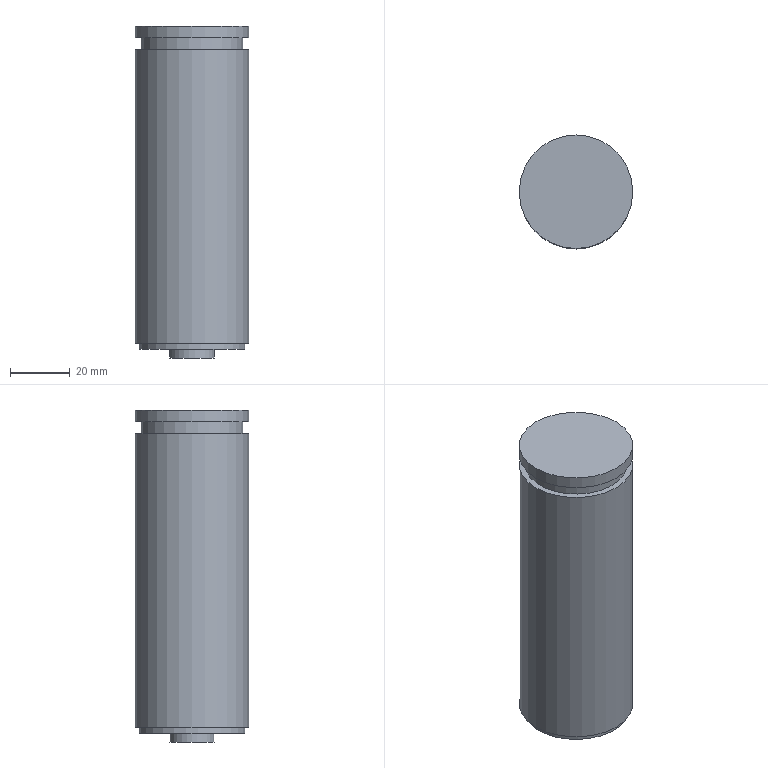Part | NX | features solid 2 | 1 solid | 11 faces | box 38 x 38 x 111 mm | volume 121810 mm3 | plane 6 | cylinder 5 | commonest cylinder face diameters 38 x2 15 x1 34 x1 35.4 x1
STEP:
#1=CARTESIAN_POINT('',(521.,-287.,289.));
#2=VERTEX_POINT('',#1);
#3=CARTESIAN_POINT('',(502.,-287.,289.));
#4=DIRECTION('',(0.,0.,1.));
#5=DIRECTION('',(1.,0.,0.));
#6=AXIS2_PLACEMENT_3D('',#3,#4,#5);
#7=CIRCLE('',#6,19.);
#8=EDGE_CURVE('',#2,#2,#7,.T.);
#9=ORIENTED_EDGE('',*,*,#8,.F.);
#10=EDGE_LOOP('',(#9));
#11=FACE_BOUND('',#10,.T.);
#12=CARTESIAN_POINT('',(519.7,-287.,289.));
#13=VERTEX_POINT('',#12);
#14=CARTESIAN_POINT('',(502.,-287.,289.));
#15=DIRECTION('',(0.,0.,1.));
#16=DIRECTION('',(1.,0.,0.));
#17=AXIS2_PLACEMENT_3D('',#14,#15,#16);
#18=CIRCLE('',#17,17.7);
#19=EDGE_CURVE('',#13,#13,#18,.F.);
#20=ORIENTED_EDGE('',*,*,#19,.F.);
#21=EDGE_LOOP('',(#20));
#22=FACE_BOUND('',#21,.T.);
#23=CARTESIAN_POINT('',(502.,-287.,289.));
#24=DIRECTION('',(0.,0.,1.));
#25=DIRECTION('',(1.,0.,0.));
#26=AXIS2_PLACEMENT_3D('',#23,#24,#25);
#27=PLANE('',#26);
#28=ADVANCED_FACE('',(#11,#22),#27,.F.);
#29=CARTESIAN_POINT('',(521.,-287.,387.));
#30=VERTEX_POINT('',#29);
#31=CARTESIAN_POINT('',(502.,-287.,387.));
#32=DIRECTION('',(0.,0.,1.));
#33=DIRECTION('',(1.,0.,0.));
#34=AXIS2_PLACEMENT_3D('',#31,#32,#33);
#35=CIRCLE('',#34,19.);
#36=EDGE_CURVE('',#30,#30,#35,.T.);
#37=ORIENTED_EDGE('',*,*,#36,.F.);
#38=EDGE_LOOP('',(#37));
#39=FACE_BOUND('',#38,.T.);
#40=ORIENTED_EDGE('',*,*,#8,.T.);
#41=EDGE_LOOP('',(#40));
#42=FACE_BOUND('',#41,.T.);
#43=CARTESIAN_POINT('',(502.,-287.,406.));
#44=DIRECTION('',(0.,0.,-1.));
#45=DIRECTION('',(-1.,0.,0.));
#46=AXIS2_PLACEMENT_3D('',#43,#44,#45);
#47=CYLINDRICAL_SURFACE('',#46,19.);
#48=ADVANCED_FACE('',(#39,#42),#47,.T.);
#49=CARTESIAN_POINT('',(509.5,-287.,287.));
#50=VERTEX_POINT('',#49);
#51=CARTESIAN_POINT('',(502.,-287.,287.));
#52=DIRECTION('',(0.,0.,1.));
#53=DIRECTION('',(1.,0.,0.));
#54=AXIS2_PLACEMENT_3D('',#51,#52,#53);
#55=CIRCLE('',#54,7.5);
#56=EDGE_CURVE('',#50,#50,#55,.T.);
#57=ORIENTED_EDGE('',*,*,#56,.T.);
#58=EDGE_LOOP('',(#57));
#59=FACE_BOUND('',#58,.T.);
#60=CARTESIAN_POINT('',(519.7,-287.,287.));
#61=VERTEX_POINT('',#60);
#62=CARTESIAN_POINT('',(502.,-287.,287.));
#63=DIRECTION('',(0.,0.,1.));
#64=DIRECTION('',(1.,0.,0.));
#65=AXIS2_PLACEMENT_3D('',#62,#63,#64);
#66=CIRCLE('',#65,17.7);
#67=EDGE_CURVE('',#61,#61,#66,.T.);
#68=ORIENTED_EDGE('',*,*,#67,.F.);
#69=EDGE_LOOP('',(#68));
#70=FACE_BOUND('',#69,.T.);
#71=CARTESIAN_POINT('',(502.,-287.,287.));
#72=DIRECTION('',(0.,0.,1.));
#73=DIRECTION('',(1.,0.,0.));
#74=AXIS2_PLACEMENT_3D('',#71,#72,#73);
#75=PLANE('',#74);
#76=ADVANCED_FACE('',(#59,#70),#75,.F.);
#77=ORIENTED_EDGE('',*,*,#67,.T.);
#78=EDGE_LOOP('',(#77));
#79=FACE_BOUND('',#78,.T.);
#80=ORIENTED_EDGE('',*,*,#19,.T.);
#81=EDGE_LOOP('',(#80));
#82=FACE_BOUND('',#81,.T.);
#83=CARTESIAN_POINT('',(502.,-287.,417.));
#84=DIRECTION('',(0.,0.,-1.));
#85=DIRECTION('',(-1.,0.,0.));
#86=AXIS2_PLACEMENT_3D('',#83,#84,#85);
#87=CYLINDRICAL_SURFACE('',#86,17.7);
#88=ADVANCED_FACE('',(#79,#82),#87,.T.);
#89=CARTESIAN_POINT('',(509.5,-287.,284.));
#90=VERTEX_POINT('',#89);
#91=CARTESIAN_POINT('',(502.,-287.,284.));
#92=DIRECTION('',(0.,0.,1.));
#93=DIRECTION('',(1.,0.,0.));
#94=AXIS2_PLACEMENT_3D('',#91,#92,#93);
#95=CIRCLE('',#94,7.5);
#96=EDGE_CURVE('',#90,#90,#95,.T.);
#97=ORIENTED_EDGE('',*,*,#96,.T.);
#98=EDGE_LOOP('',(#97));
#99=FACE_BOUND('',#98,.T.);
#100=ORIENTED_EDGE('',*,*,#56,.F.);
#101=EDGE_LOOP('',(#100));
#102=FACE_BOUND('',#101,.T.);
#103=CARTESIAN_POINT('',(502.,-287.,285.));
#104=DIRECTION('',(0.,0.,1.));
#105=DIRECTION('',(1.,0.,0.));
#106=AXIS2_PLACEMENT_3D('',#103,#104,#105);
#107=CYLINDRICAL_SURFACE('',#106,7.5);
#108=ADVANCED_FACE('',(#99,#102),#107,.T.);
#109=ORIENTED_EDGE('',*,*,#96,.F.);
#110=EDGE_LOOP('',(#109));
#111=FACE_BOUND('',#110,.T.);
#112=CARTESIAN_POINT('',(502.,-287.,284.));
#113=DIRECTION('',(0.,0.,1.));
#114=DIRECTION('',(1.,0.,0.));
#115=AXIS2_PLACEMENT_3D('',#112,#113,#114);
#116=PLANE('',#115);
#117=ADVANCED_FACE('',(#111),#116,.F.);
#118=CARTESIAN_POINT('',(519.,-287.,391.));
#119=VERTEX_POINT('',#118);
#120=CARTESIAN_POINT('',(502.,-287.,391.));
#121=DIRECTION('',(0.,0.,1.));
#122=DIRECTION('',(1.,0.,0.));
#123=AXIS2_PLACEMENT_3D('',#120,#121,#122);
#124=CIRCLE('',#123,17.);
#125=EDGE_CURVE('',#119,#119,#124,.T.);
#126=ORIENTED_EDGE('',*,*,#125,.F.);
#127=EDGE_LOOP('',(#126));
#128=FACE_BOUND('',#127,.T.);
#129=CARTESIAN_POINT('',(519.,-287.,387.));
#130=VERTEX_POINT('',#129);
#131=CARTESIAN_POINT('',(502.,-287.,387.));
#132=DIRECTION('',(0.,0.,1.));
#133=DIRECTION('',(1.,0.,0.));
#134=AXIS2_PLACEMENT_3D('',#131,#132,#133);
#135=CIRCLE('',#134,17.);
#136=EDGE_CURVE('',#130,#130,#135,.T.);
#137=ORIENTED_EDGE('',*,*,#136,.T.);
#138=EDGE_LOOP('',(#137));
#139=FACE_BOUND('',#138,.T.);
#140=CARTESIAN_POINT('',(502.,-287.,387.));
#141=DIRECTION('',(0.,0.,1.));
#142=DIRECTION('',(1.,0.,0.));
#143=AXIS2_PLACEMENT_3D('',#140,#141,#142);
#144=CYLINDRICAL_SURFACE('',#143,17.);
#145=ADVANCED_FACE('',(#128,#139),#144,.T.);
#146=ORIENTED_EDGE('',*,*,#136,.F.);
#147=EDGE_LOOP('',(#146));
#148=FACE_BOUND('',#147,.T.);
#149=ORIENTED_EDGE('',*,*,#36,.T.);
#150=EDGE_LOOP('',(#149));
#151=FACE_BOUND('',#150,.T.);
#152=CARTESIAN_POINT('',(502.,-287.,387.));
#153=DIRECTION('',(0.,0.,-1.));
#154=DIRECTION('',(-1.,0.,0.));
#155=AXIS2_PLACEMENT_3D('',#152,#153,#154);
#156=PLANE('',#155);
#157=ADVANCED_FACE('',(#148,#151),#156,.F.);
#158=ORIENTED_EDGE('',*,*,#125,.T.);
#159=EDGE_LOOP('',(#158));
#160=FACE_BOUND('',#159,.T.);
#161=CARTESIAN_POINT('',(521.,-287.,391.));
#162=VERTEX_POINT('',#161);
#163=CARTESIAN_POINT('',(502.,-287.,391.));
#164=DIRECTION('',(0.,0.,1.));
#165=DIRECTION('',(1.,0.,0.));
#166=AXIS2_PLACEMENT_3D('',#163,#164,#165);
#167=CIRCLE('',#166,19.);
#168=EDGE_CURVE('',#162,#162,#167,.T.);
#169=ORIENTED_EDGE('',*,*,#168,.F.);
#170=EDGE_LOOP('',(#169));
#171=FACE_BOUND('',#170,.T.);
#172=CARTESIAN_POINT('',(502.,-287.,391.));
#173=DIRECTION('',(0.,0.,-1.));
#174=DIRECTION('',(-1.,0.,0.));
#175=AXIS2_PLACEMENT_3D('',#172,#173,#174);
#176=PLANE('',#175);
#177=ADVANCED_FACE('',(#160,#171),#176,.T.);
#178=CARTESIAN_POINT('',(521.,-287.,395.));
#179=VERTEX_POINT('',#178);
#180=CARTESIAN_POINT('',(502.,-287.,395.));
#181=DIRECTION('',(0.,0.,1.));
#182=DIRECTION('',(1.,0.,0.));
#183=AXIS2_PLACEMENT_3D('',#180,#181,#182);
#184=CIRCLE('',#183,19.);
#185=EDGE_CURVE('',#179,#179,#184,.T.);
#186=ORIENTED_EDGE('',*,*,#185,.T.);
#187=EDGE_LOOP('',(#186));
#188=FACE_BOUND('',#187,.T.);
#189=CARTESIAN_POINT('',(502.,-287.,395.));
#190=DIRECTION('',(0.,0.,1.));
#191=DIRECTION('',(1.,0.,0.));
#192=AXIS2_PLACEMENT_3D('',#189,#190,#191);
#193=PLANE('',#192);
#194=ADVANCED_FACE('',(#188),#193,.T.);
#195=ORIENTED_EDGE('',*,*,#168,.T.);
#196=EDGE_LOOP('',(#195));
#197=FACE_BOUND('',#196,.T.);
#198=ORIENTED_EDGE('',*,*,#185,.F.);
#199=EDGE_LOOP('',(#198));
#200=FACE_BOUND('',#199,.T.);
#201=CARTESIAN_POINT('',(502.,-287.,406.));
#202=DIRECTION('',(0.,0.,-1.));
#203=DIRECTION('',(-1.,0.,0.));
#204=AXIS2_PLACEMENT_3D('',#201,#202,#203);
#205=CYLINDRICAL_SURFACE('',#204,19.);
#206=ADVANCED_FACE('',(#197,#200),#205,.T.);
#207=CLOSED_SHELL('',(#28,#48,#76,#88,#108,#117,#145,#157,#177,#194,#206));
#208=MANIFOLD_SOLID_BREP('',#207);
#209=(LENGTH_UNIT()NAMED_UNIT(*)SI_UNIT(.MILLI.,.METRE.));
#210=UNCERTAINTY_MEASURE_WITH_UNIT(LENGTH_MEASURE(0.00001),#209,'','');
#211=(NAMED_UNIT(*)PLANE_ANGLE_UNIT()SI_UNIT($,.RADIAN.));
#212=(NAMED_UNIT(*)SI_UNIT($,.STERADIAN.)SOLID_ANGLE_UNIT());
#213=(GEOMETRIC_REPRESENTATION_CONTEXT(3)GLOBAL_UNCERTAINTY_ASSIGNED_CONTEXT((#210))GLOBAL_UNIT_ASSIGNED_CONTEXT((#209,#211,#212))REPRESENTATION_CONTEXT('',''));
#214=ADVANCED_BREP_SHAPE_REPRESENTATION('',(#208),#213);